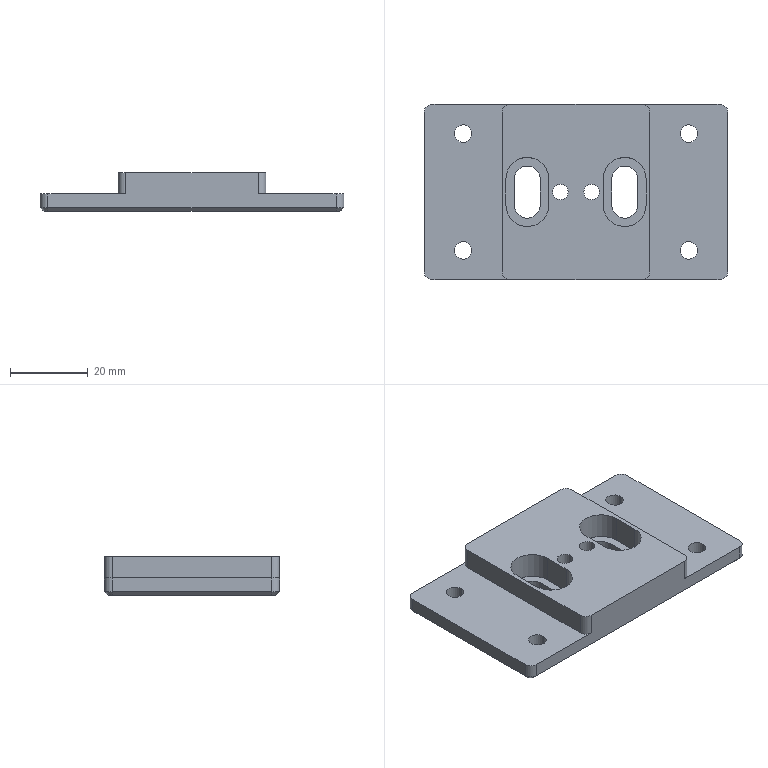NC program | NX | posted with a generic post | part box 78 x 45 x 10 mm
Lines 1 to 1682 of 4289, first 1506 of 1672 lines:
N10 G17 G21 G94 G90
(FLOOR_WALL , TOOL : D63)
N12 T01 M6
N14 G54
N16 G17 G0 G90 X-76.5 Y0. S6500 M3
N18 G43 Z30. H1
N20 Z3.
N22 G94 G1 Z0. F1250.
N24 X-73.5
N26 X73.5
N28 X76.5
N30 Z3.
N32 G0 Z30.
N34 M5
(ADAPTIVE_MILLING , TOOL : D10)
N36 T10 M6
N38 G54
N40 G17 G0 G90 X-49.696 Y-0.05 S9500 M3
N42 G43 Z30. H10
N44 Z-9.
N46 G94 G1 Z-10. F1000.
N48 X-48.34 Y-0.58 F3000.
N50 G3 X-47.049 Y-0.05 R1.015
N52 X-46.406 Y3.11 R9.424
N54 X-46.21 Y14.606 R185.073
N56 G2 X-46.176 Y23.305 R429.662
N58 X-43.276 Y27.539 R6.067
N60 X-37.706 Y29.327 R13.136
N62 X-29.118 Y29.675 R79.661
N64 G1 X-27.618 Y29.682
N66 X-25.518 Y29.687
N68 X-21.918 Y29.69
N70 X-8.218 Y29.691
N72 X39.282
N74 X39.382 Y29.689
N76 G2 X43.858 Y27.028 R5.824
N78 X45.771 Y21.61 R12.335
N80 X46.17 Y13.325 R66.724
N82 G1 X46.178 Y12.025
N84 X46.184 Y10.325
N86 X46.188 Y7.825
N88 X46.19 Y2.725
N90 Y-22.775
N92 Y-22.875
N94 G2 X43.535 Y-27.355 R5.815
N96 X38.118 Y-29.271 R12.321
N98 X30.134 Y-29.668 R64.412
N100 G1 X28.934 Y-29.676
N102 X27.334 Y-29.683
N104 X25.134 Y-29.687
N106 X21.234 Y-29.69
N108 X-0.766 Y-29.691
N110 X-39.266
N112 G2 X-43.609 Y-27.362 R5.645
N114 X-45.71 Y-22.022 R11.517
N116 X-46.166 Y-13.843 R57.666
N118 X-46.15 Y-2.344 R358.837
N120 G3 X-45.434 Y11.629 R117.265
N122 G1 X-45.426 Y13.229
N124 X-45.421 Y15.429
N126 X-45.418 Y18.929
N128 X-45.417 Y20.029
N130 X-45.414 Y20.229
N132 X-45.406 Y20.429
N134 X-45.4 Y20.529
N136 X-45.393 Y20.629
N138 G2 X-41.395 Y26.625 R7.729
N140 X-35.115 Y28.496 R16.062
N142 X-25.726 Y28.865 R92.161
N144 G1 X-24.226 Y28.872
N146 X-22.127 Y28.877
N148 X-18.827 Y28.88
N150 X-10.427 Y28.882
N152 X36.473
N154 X36.673 Y28.88
N156 G2 X42.939 Y25.168 R7.555
N158 X44.964 Y18.84 R15.167
N160 X45.363 Y9.553 R83.82
N162 G1 X45.37 Y8.053
N164 X45.376 Y6.053
N166 X45.38 Y3.053
N168 X45.381 Y-3.547
N170 X45.382 Y-20.047
N172 X45.381 Y-20.147
N174 G2 X41.606 Y-26.479 R7.587
N176 X35.465 Y-28.45 R15.175
N178 X25.98 Y-28.863 R83.109
N180 G1 X24.48 Y-28.87
N182 X22.48 Y-28.876
N184 X19.38 Y-28.88
N186 X12.88 Y-28.882
N188 X-36.52
N190 X-36.62 Y-28.881
N192 G2 X-42.965 Y-25.128 R7.577
N194 X-44.973 Y-18.793 R15.322
N196 X-45.363 Y-9.507 R85.57
N198 X-44.961 Y1.679 R97.942
N200 G3 X-44.625 Y17.873 R263.26
N202 G2 X-44.092 Y21.014 R9.947
N204 G1 X-43.977 Y22.032
N206 X-43.951 Y22.147
N208 G2 X-41.5 Y26.048 R7.672
N210 X-38.532 Y27.477 R8.031
N212 X-29.579 Y27.987 R94.219
N214 X-10.679 Y28.073 R882.599
N216 G1 X34.221
N218 X34.421 Y28.07
N220 X34.621 Y28.066
N222 X34.821 Y28.058
N224 X34.92 Y28.053
N226 G2 X37.322 Y27.614 R10.194
N228 X40.152 Y26.911 R7.665
N230 X43.411 Y23.652 R7.672
N232 X44.147 Y20.529 R8.254
N234 X44.569 Y2.779 R255.07
N236 G1 X44.572 Y-1.521
N238 X44.573 Y-15.521
N240 Y-17.721
N242 X44.57 Y-17.921
N244 X44.566 Y-18.121
N246 X44.558 Y-18.32
N248 G2 X44.115 Y-20.813 R10.023
N250 X43.411 Y-23.652 R7.679
N252 X40.152 Y-26.911 R7.672
N254 X37.029 Y-27.647 R8.254
N256 X21.179 Y-28.065 R231.381
N258 G1 X18.379 Y-28.07
N260 X13.379 Y-28.073
N262 X-25.221
N264 X-34.221
N266 X-34.421 Y-28.07
N268 X-34.621 Y-28.066
N270 G2 X-37.314 Y-27.615 R9.926
N272 X-40.152 Y-26.911 R7.678
N274 X-43.411 Y-23.652 R7.672
N276 X-44.147 Y-20.529 R8.254
N278 X-44.434 Y-2.882 R158.962
N280 G1 X-44.393 Y-2.183
N282 X-44.326 Y-1.085
N284 X-44.275 Y-0.287
N286 X-44.223 Y0.612
N288 X-44.157 Y1.81
N290 X-44.15 Y1.934
N292 Y20.471
N294 X-44.147 Y20.529
N296 X-44.091 Y21.026
N298 X-44.033 Y21.588
N300 X-43.951 Y22.147
N302 G2 X-41.5 Y26.048 R7.672
N304 X-38.532 Y27.477 R8.031
N306 G1 X-36.971 Y27.65
N308 X36.971
N310 X37.029 Y27.647
N312 X37.327 Y27.613
N314 G2 X40.152 Y26.911 R7.657
N316 X43.411 Y23.652 R7.672
N318 G1 X43.461 Y23.547
N320 X43.951 Y22.147
N322 X43.977 Y22.032
N324 X44.15 Y20.471
N326 Y-20.471
N328 X44.147 Y-20.529
N330 X44.113 Y-20.827
N332 G2 X43.411 Y-23.652 R7.657
N334 X40.152 Y-26.911 R7.672
N336 G1 X40.047 Y-26.961
N338 X38.647 Y-27.451
N340 X38.532 Y-27.477
N342 X36.971 Y-27.65
N344 X-36.971
N346 X-37.029 Y-27.647
N348 X-37.327 Y-27.613
N350 G2 X-40.152 Y-26.911 R7.657
N352 X-43.411 Y-23.652 R7.672
N354 G1 X-43.461 Y-23.547
N356 X-43.951 Y-22.147
N358 X-43.977 Y-22.032
N360 X-44.15 Y-20.471
N362 Y2.029
N364 G3 X-45.004 Y3.027 R1.016
N366 G1 X-46.57 Y3.271
N368 Z-7.
N370 G0 Z30.
N372 X-17.027 Y-30.147
N374 Z-4.349
N376 G1 Z-5.349 F1000.
N378 X-16.915 Y-29.348 F3000.
N380 X-16.827 Y-28.545
N382 G3 X-17.723 Y-27.569 R1.015
N384 G2 X-19.815 Y-27.183 R16.236
N386 G3 X-27.301 Y-26.829 R57.109
N388 G2 X-35.5 Y-26.768 R358.172
N390 X-41.868 Y-22.187 R7.175
N392 X-43.108 Y-16.042 R18.598
N394 X-43.29 Y-2.345 R262.741
N396 G1 X-43.291 Y10.755
N398 Y17.855
N400 X-43.288 Y18.155
N402 X-43.281 Y18.455
N404 X-43.274 Y18.655
N406 G2 X-38.625 Y25.388 R7.203
N408 X-32.576 Y26.607 R18.677
N410 X-20.479 Y26.805 R249.647
N412 G1 X-20.381 Y26.824
N414 X-20.285 Y26.852
N416 X-20.191 Y26.886
N418 X-20.152 Y26.911
N420 X-20.047 Y26.961
N422 X-18.647 Y27.451
N424 X-18.532 Y27.477
N426 X-17.638 Y27.578
N428 G3 X-17.737 Y29.573 R1.001
N430 G1 X-19.732 Y29.708 Z-5.249
N432 X-21.535 Y29.828
N434 X-30.91
N436 G3 X-37.067 Y29.07 R25.605
N438 G1 X-39.365 Y28.483
N440 G3 X-42.229 Y27.036 R8.814
N442 G1 X-42.693 Y26.628
N444 X-43.125 Y26.186
N446 X-44.628 Y24.467
N448 G3 X-45.923 Y21.531 R6.624
N450 X-46.251 Y17.815 R23.796
N452 G1 X-46.469 Y-12.529
N454 G3 X-45.306 Y-21.924 R37.581
N456 X-42.558 Y-26.649 R10.739
N458 G1 X-41.378 Y-27.811
N460 G3 X-38.52 Y-29.278 R6.575
N462 X-34.822 Y-29.815 R23.711
N464 G1 X-21.829 Y-30.633
N466 X-21.59 Y-30.616
N468 X-21.36 Y-30.549
N470 X-19.622 Y-29.777
N472 X-19.017 Y-29.513 Z-5.282
N474 X-18.422 Y-29.227 Z-5.315
N476 G3 X-18.023 Y-28.694 Z-5.349 R1.039
N478 X-18.647 Y-27.451 R1.005
N480 X-24.663 Y-26.187 R16.875
N482 X-33.56 Y-25.986 R419.368
N484 G2 X-40.311 Y-21.648 R8.075
N486 X-42.123 Y-15.246 R16.696
N488 X-42.473 Y-4.356 R113.695
N490 G1 X-42.478 Y-2.156
N492 X-42.481 Y1.544
N494 X-42.482 Y12.844
N496 Y15.944
N498 X-42.48 Y16.144
N500 X-42.478 Y16.344
N502 G2 X-37.96 Y23.901 R8.152
N504 X-31.436 Y25.655 R17.356
N506 X-22.245 Y25.989 R121.545
N508 G3 X-21.366 Y26.148 R2.601
N510 G1 X-20.181 Y26.893
N512 G3 X-19.876 Y28.287 R1.004
N514 X-20.781 Y28.754 Z-5.296 R1.115
N516 G1 X-21.714 Y28.866 Z-5.249
N518 X-24.078 Y29.143
N520 X-27.576 Y29.128
N522 G3 X-31.55 Y28.771 R34.824
N524 G1 X-34.142 Y28.367
N526 G3 X-38.741 Y26.858 R17.997
N528 G1 X-39.56 Y26.412
N530 X-40.354 Y25.922
N532 X-41.525 Y25.151
N534 X-42.68 Y24.357
N536 G3 X-43.753 Y22.981 R4.397
N538 G1 X-44.211 Y21.983
N540 X-44.643 Y20.975
N542 G3 X-45.305 Y17.878 R10.422
N544 G1 X-45.55 Y13.201
N546 X-45.736 Y8.52
N548 X-46.049 Y-1.477
N550 G3 X-45.387 Y-13.915 R74.276
N552 G1 X-44.7 Y-18.867
N554 G3 X-43.334 Y-22.574 R9.795
N556 G1 X-42.783 Y-23.403
N558 X-41.307 Y-25.411
N560 G3 X-40.231 Y-26.531 R6.738
N562 X-37.274 Y-28.244 R14.155
N564 X-34.876 Y-28.858 R9.068
N566 G1 X-23.229 Y-30.143
N568 G3 X-22.68 Y-30.048 R1.055
N570 G1 X-21.077 Y-29.266
N572 X-20.481 Y-28.981 Z-5.282
N574 X-19.897 Y-28.674 Z-5.315
N576 G3 X-19.516 Y-28.128 Z-5.349 R1.039
N578 X-20.047 Y-26.961 R1.007
N580 X-23.812 Y-25.676 R8.467
N582 X-31.295 Y-25.249 R69.666
N584 G2 X-39.48 Y-20.075 R9.177
N586 X-41.301 Y-13.256 R18.936
N588 X-41.661 Y-2.366 R118.207
N590 X-41.64 Y15.333 R923.775
N592 X-36.575 Y22.959 R9.056
N594 X-29.763 Y24.798 R18.711
N596 X-23.176 Y25.191 R200.74
N598 G3 X-21.5 Y26.048 R2.091
N600 G1 X-21.408 Y26.121
N602 X-21.323 Y26.175
N604 G3 X-21.009 Y27.553 R1.004
N606 X-21.92 Y28.036 Z-5.295 R1.109
N608 G1 X-22.838 Y28.146 Z-5.249
N610 X-25.22 Y28.425
N612 X-26.344 Y28.426
N614 X-27.466 Y28.385
N616 X-28.209 Y28.3
N618 X-28.946 Y28.18
N620 X-31.459 Y27.681
N622 X-33.967 Y27.161
N624 G3 X-38.298 Y25.602 R22.076
N626 X-41.392 Y23.152 R9.534
N628 G1 X-42.312 Y22.023
N630 X-43.214 Y20.88
N632 G3 X-44.07 Y19.032 R5.959
N634 X-44.547 Y15.96 R16.463
N636 G1 X-44.67 Y14.092
N638 X-44.736 Y12.222
N640 X-45.007 Y-5.279
N642 G3 X-44.37 Y-13.971 R49.652
N644 G1 X-43.942 Y-16.521
N646 G3 X-42.484 Y-21.098 R21.242
N648 X-39.929 Y-24.623 R11.844
N650 G1 X-38.65 Y-25.812
N652 G3 X-36.084 Y-27.305 R9.328
N654 X-32.213 Y-28.203 R13.677
N656 G1 X-24.454 Y-28.845
N658 X-22.235 Y-28.575
N660 X-21.57 Y-28.497 Z-5.283
N662 X-20.908 Y-28.397 Z-5.316
N664 G3 X-20.379 Y-28.021 Z-5.349 R1.041
N666 X-20.66 Y-26.591 R1.004
N668 X-25.088 Y-24.933 R9.128
N670 X-30.566 Y-24.46 R108.938
N672 G2 X-38.695 Y-18.59 R10.05
N674 X-40.481 Y-11.551 R20.915
N676 X-40.847 Y-0.961 R119.577
N678 X-40.828 Y13.639 R749.065
N680 X-35.279 Y22.066 R9.806
N682 X-28.071 Y23.977 R20.186
N684 G3 X-23.597 Y24.439 R61.952
N686 X-22.548 Y25. R1.508
N688 G1 X-21.983 Y25.565
N690 G3 X-21.811 Y26.749 R1.007
N692 X-22.687 Y27.289 Z-5.295 R1.11
N694 G1 X-23.598 Y27.46 Z-5.249
N696 X-25.626 Y27.833
N698 X-25.88 Y27.815
N700 X-29.005 Y27.196
N702 X-32.126 Y26.552
N704 G3 X-37.733 Y24.215 R18.405
N706 X-41.371 Y20.86 R14.166
N708 X-43.398 Y16.387 R9.938
N710 X-43.956 Y12.064 R33.416
N712 X-44.196 Y4.204 R96.24
N714 G1 X-44.158 Y2.707
N716 X-43.745 Y-9.164
N718 G3 X-42.963 Y-15.338 R34.55
N720 G1 X-42.714 Y-16.469
N722 X-42.419 Y-17.588
N724 G3 X-40.984 Y-20.659 R13.498
N726 X-38.929 Y-23.511 R23.056
N728 X-34.108 Y-26.687 R11.409
N730 G1 X-33.152 Y-26.973
N732 X-32.183 Y-27.209
N734 X-30.81 Y-27.492
N736 X-29.429 Y-27.734
N738 X-25.305 Y-28.371
N740 X-25. Y-28.372
N742 X-23.018 Y-28.067
N744 X-22.364 Y-27.971 Z-5.282
N746 X-21.715 Y-27.852 Z-5.315
N748 G3 X-21.189 Y-27.443 Z-5.349 R1.039
N750 X-21.408 Y-26.121 R1.005
N752 X-24.384 Y-24.546 R5.831
N754 X-29.222 Y-23.792 R43.916
N756 G2 X-37.913 Y-17.225 R10.96
N758 X-39.716 Y-9.471 R23.407
N760 X-40.047 Y3.221 R166.788
N762 X-39.993 Y12.419 R204.804
N764 X-33.895 Y21.278 R10.435
N766 X-27.467 Y23.062 R21.125
N768 G3 X-23.741 Y23.771 R19.944
N770 X-23.049 Y24.227 R1.57
N772 G1 X-22.624 Y24.904
N774 G3 X-22.583 Y25.898 R1.014
N776 X-23.301 Y26.427 Z-5.303 R1.049
N778 G1 X-24.341 Y26.712 Z-5.249
N780 X-26.109 Y27.187
N782 X-26.316 Y27.188
N784 X-26.521 Y27.154
N786 G3 X-30.978 Y25.741 R69.932
N788 G1 X-32.58 Y25.122
N790 X-34.175 Y24.486
N792 G3 X-38.369 Y21.861 R17.493
N794 X-41.461 Y18.249 R12.617
N796 X-42.583 Y15.188 R11.04
N798 X-42.98 Y12.104 R18.094
N800 G1 X-43.397 Y1.488
N802 G3 X-42.983 Y-8.471 R62.231
N804 G1 X-42.74 Y-10.432
N806 X-42.441 Y-12.386
N808 G3 X-41.108 Y-17.622 R43.62
N810 X-35.439 Y-24.718 R12.319
N812 X-32.897 Y-25.872 R16.542
N814 G1 X-31.571 Y-26.33
N816 X-30.229 Y-26.74
N818 X-25.68 Y-28.016
N820 X-25.448 Y-28.048
N822 X-25.215 Y-28.034
N824 X-23.424 Y-27.678
N826 X-22.776 Y-27.554 Z-5.282
N828 X-22.132 Y-27.407 Z-5.315
N830 G3 X-21.625 Y-26.975 Z-5.349 R1.039
N832 X-21.782 Y-25.766 R1.007
N834 X-25.109 Y-23.855 R6.221
N836 G2 X-29.399 Y-22.885 R291.286
N838 X-37.231 Y-15.726 R11.907
N840 X-38.909 Y-7.938 R25.813
N842 X-39.237 Y4.755 R174.442
N844 X-39.135 Y11.452 R80.404
N846 X-32.778 Y20.395 R10.909
N848 X-26.672 Y22.251 R25.621
N850 G3 X-23.822 Y23.153 R10.905
N852 X-23.411 Y23.652 R1.541
N854 G1 X-23.038 Y24.245
N856 G3 X-23.167 Y25.473 R1.007
N858 X-24.087 Y25.761 Z-5.299 R1.037
N860 G1 X-25.079 Y25.659 Z-5.249
N862 X-26.233 Y25.544
N864 X-27.385 Y25.41
N866 X-29.021 Y25.002
N868 X-30.645 Y24.549
N870 G3 X-36.058 Y22.043 R21.755
N872 X-38.841 Y19.587 R13.102
N874 G1 X-40.311 Y17.835
N876 G3 X-41.474 Y15.434 R7.556
N878 G1 X-41.71 Y14.53
N880 X-41.889 Y13.613
N882 G3 X-42.385 Y8.164 R32.733
N884 G1 X-42.39 Y3.246
N886 X-42.37 Y-1.672
N888 G3 X-41.847 Y-8.932 R72.751
N890 G1 X-41.5 Y-11.615
N892 G3 X-40.078 Y-16.807 R23.581
N894 X-37.9 Y-20.548 R17.726
N896 X-32.097 Y-25.065 R13.364
N898 G1 X-26.245 Y-27.45
N900 G3 X-25.654 Y-27.501 R1.048
N902 G1 X-23.984 Y-27.134
N904 X-23.331 Y-26.996 Z-5.282
N906 X-22.683 Y-26.835 Z-5.316
N908 G3 X-22.19 Y-26.408 Z-5.349 R1.04
N910 X-22.348 Y-25.2 R1.007
N912 X-25.324 Y-23.284 R5.749
N914 G2 X-29.769 Y-21.768 R41.624
N916 X-36.592 Y-14.162 R13.057
N918 X-38.146 Y-5.936 R29.445
N920 X-38.367 Y9.557 R187.76
N922 X-31.819 Y19.472 R11.374
N924 X-26.749 Y21.308 R30.248
N926 G3 X-24.004 Y22.482 R9.19
N928 X-23.461 Y23.547 R2.228
N930 X-23.673 Y24.558 R1.011
N932 X-24.526 Y24.874 Z-5.302 R1.046
N934 G1 X-25.583 Y24.848 Z-5.249
N936 X-27.549 Y24.79
N938 X-27.808 Y24.711
N940 X-30.647 Y23.408
N942 X-33.478 Y22.088
N944 G3 X-37.357 Y19.405 R17.782
N946 X-39.031 Y17.25 R10.785
N948 X-40.513 Y14.124 R17.41
N950 X-41.089 Y11.444 R13.822
N952 X-41.759 Y3.778 R69.955
N954 X-41.645 Y-0.378 R44.213
N956 G1 X-41.354 Y-4.22
N958 X-41.044 Y-8.061
N960 G3 X-39.786 Y-14.202 R33.376
N962 X-37.127 Y-19.529 R18.595
N964 G1 X-36.447 Y-20.461
N966 X-35.727 Y-21.364
N968 G3 X-30.472 Y-24.857 R12.476
N970 G1 X-26.855 Y-26.105
N972 X-24.694 Y-26.324
N974 X-24.045 Y-26.394 Z-5.282
N976 X-23.393 Y-26.437 Z-5.314
N978 G3 X-22.773 Y-26.159 Z-5.349 R1.038
N980 X-22.621 Y-24.908 R1.007
N982 X-24.849 Y-22.984 R4.491
N984 G2 X-29.133 Y-21.054 R82.148
N986 X-35.88 Y-12.831 R14.312
N988 X-37.372 Y-4.085 R33.221
N990 X-37.529 Y8.509 R131.827
N992 X-31.207 Y18.413 R11.761
N994 X-26.263 Y20.573 R45.314
N996 G3 X-24.121 Y21.826 R6.281
N998 X-23.687 Y22.902 R4.923
N1000 X-23.935 Y23.95 R1.011
N1002 X-24.827 Y24.231 Z-5.301 R1.135
N1004 G1 X-25.861 Y24.222 Z-5.249
N1006 X-27.66 Y24.199
N1008 X-27.852 Y24.148
N1010 X-28.034 Y24.066
N1012 X-30.484 Y22.601
N1014 X-32.924 Y21.118
N1016 G3 X-37.373 Y17.197 R21.29
N1018 X-39.142 Y14.3 R12.771
N1020 X-40.463 Y10.289 R18.335
N1022 X-40.683 Y7.82 R13.498
N1024 G1 X-40.608 Y-2.805
N1026 G3 X-39.795 Y-10.221 R36.9
N1028 G1 X-39.514 Y-11.527
N1030 X-39.186 Y-12.822
N1032 G3 X-36.027 Y-19.135 R18.99
N1034 X-31.123 Y-23.411 R16.313
N1036 G1 X-27.287 Y-25.565
N1038 X-27.088 Y-25.646
N1040 X-26.877 Y-25.69
N1042 X-25.008 Y-25.838
N1044 X-24.353 Y-25.896 Z-5.282
N1046 X-23.696 Y-25.928 Z-5.315
N1048 G3 X-23.087 Y-25.646 Z-5.349 R1.039
N1050 X-22.941 Y-24.4 R1.007
N1052 X-25.17 Y-22.312 R5.279
N1054 G2 X-29.623 Y-19.637 R39.755
N1056 X-35.375 Y-10.849 R16.112
N1058 X-36.63 Y-1.554 R41.35
N1060 X-36.682 Y7.542 R87.595
N1062 X-30.562 Y17.413 R12.271
N1064 X-25.958 Y19.827 R78.966
N1066 G3 X-24.153 Y21.216 R5.
N1068 X-23.955 Y22.13 R3.206
N1070 X-24.402 Y23.202 R1.007
N1072 X-25.363 Y23.259 Z-5.299 R1.037
N1074 G1 X-26.302 Y22.921 Z-5.249
N1076 X-28.305 Y22.199
N1078 X-28.455 Y22.13
N1080 X-29.923 Y21.307
N1082 X-31.37 Y20.449
N1084 G3 X-35.628 Y17.2 R30.221
N1086 X-38.354 Y13.086 R10.962
N1088 X-39.439 Y8.893 R16.044
N1090 G1 X-39.907 Y4.547
N1092 X-40.004 Y3.302
N1094 X-40.042 Y2.055
N1096 X-40.017 Y1.432
N1098 X-39.976 Y0.809
N1100 X-39.617 Y-3.056
N1102 X-39.237 Y-6.92
N1104 G3 X-37.902 Y-13.013 R34.9
N1106 X-35.574 Y-17.837 R17.228
N1108 X-32.505 Y-21.26 R18.589
N1110 G1 X-31.65 Y-21.987
N1112 X-30.768 Y-22.683
N1114 X-27.607 Y-25.057
N1116 G3 X-27.064 Y-25.255 R1.051
N1118 G1 X-25.316 Y-25.356
N1120 X-24.656 Y-25.399 Z-5.282
N1122 X-23.995 Y-25.418 Z-5.315
N1124 G3 X-23.397 Y-25.129 Z-5.349 R1.039
N1126 X-23.26 Y-23.892 R1.007
N1128 X-25.339 Y-21.645 R5.766
N1130 G2 X-29.926 Y-18.109 R34.106
N1132 X-34.801 Y-8.973 R18.311
N1134 X-35.871 Y0.953 R51.581
N1136 X-35.699 Y7.642 R37.584
N1138 X-30.3 Y16.19 R12.703
N1140 X-25.816 Y19.011 R103.195
N1142 G3 X-24.207 Y20.482 R4.979
N1144 X-24.022 Y21.637 R5.423
N1146 X-24.525 Y22.62 R1.01
N1148 X-25.409 Y22.674 Z-5.303 R1.049
N1150 G1 X-26.443 Y22.349 Z-5.249
N1152 X-28.221 Y21.791
N1154 X-28.376 Y21.723
N1156 X-28.522 Y21.637
N1158 X-33.024 Y18.26
N1160 G3 X-36.831 Y13.552 R12.433
N1162 X-38.83 Y7.587 R24.313
N1164 X-39.141 Y3.35 R19.584
N1166 G1 X-38.951 Y-1.468
N1168 G3 X-37.503 Y-10.667 R51.208
N1170 X-34.38 Y-17.544 R22.835
N1172 G1 X-33.611 Y-18.612
N1174 X-32.825 Y-19.667
N1176 G3 X-29.889 Y-22.307 R12.475
N1178 G1 X-27.874 Y-23.597
N1180 X-25.82 Y-24.4
N1182 X-25.215 Y-24.641 Z-5.282
N1184 X-24.6 Y-24.858 Z-5.314
N1186 G3 X-23.926 Y-24.755 Z-5.349 R1.038
N1188 X-23.461 Y-23.547 R1.006
N1190 X-25.046 Y-21.287 R4.825
N1192 G2 X-29.12 Y-17.596 R61.317
N1194 X-34.108 Y-7.514 R20.263
N1196 X-34.975 Y5.524 R54.962
N1198 X-29.682 Y15.237 R13.473
N1200 X-25.573 Y18.255 R540.304
N1202 G3 X-24.224 Y19.71 R4.816
N1204 X-24.113 Y20.827 R6.496
N1206 X-24.608 Y21.806 R1.01
N1208 X-25.483 Y21.871 Z-5.304 R1.051
N1210 G1 X-26.533 Y21.564 Z-5.249
N1212 X-28.187 Y21.08
N1214 X-28.414 Y20.977
N1216 X-28.613 Y20.827
N1218 X-33.474 Y15.966
N1220 G3 X-37.663 Y7.814 R14.761
N1222 G1 X-37.79 Y6.891
N1224 X-37.873 Y5.963
N1226 X-38.103 Y1.776
N1228 G3 X-37.766 Y-4.615 R38.997
N1230 X-37.155 Y-8.308 R42.153
N1232 X-35.826 Y-12.724 R33.038
N1234 X-32.826 Y-17.868 R19.631
N1236 G1 X-31.617 Y-19.297
N1238 X-30.363 Y-20.688
N1240 X-28.127 Y-23.075
N1242 X-27.944 Y-23.224
N1244 X-27.735 Y-23.332
N1246 X-25.974 Y-23.964
N1248 X-25.361 Y-24.189 Z-5.282
N1250 X-24.741 Y-24.39 Z-5.314
N1252 G3 X-24.071 Y-24.271 Z-5.349 R1.038
N1254 X-23.627 Y-23.075 R1.007
N1256 X-25.365 Y-20.313 R6.434
N1258 G2 X-29.493 Y-15.696 R44.517
N1260 X-33.502 Y-5.561 R23.486
N1262 X-34.086 Y4.7 R44.881
N1264 X-29.241 Y14.162 R14.154
N1266 G1 X-25.285 Y17.534
N1268 G3 X-24.192 Y18.945 R4.197
N1270 X-24.15 Y20.065 R7.43
N1272 X-24.884 Y21.029 R1.007
N1274 X-25.882 Y20.77 Z-5.295 R1.109
N1276 G1 X-26.635 Y20.232 Z-5.249
N1278 X-28.073 Y19.201
N1280 X-29.537 Y18.207
N1282 G3 X-31.423 Y16.593 R10.707
N1284 G1 X-33.445 Y14.38
N1286 G3 X-35.697 Y10.526 R12.964
N1288 X-36.866 Y6.34 R20.982
N1290 G1 X-37.172 Y4.491
N1292 X-37.446 Y2.637
N1294 G3 X-37.46 Y1.394 R6.405
N1296 G1 X-37.201 Y-1.28
N1298 X-36.924 Y-3.952
N1300 G3 X-35.507 Y-10.271 R32.676
N1302 X-31.569 Y-18.023 R31.925
N1304 G1 X-30.485 Y-19.548
N1306 X-28.358 Y-22.414
N1308 G3 X-27.874 Y-22.766 R1.047
N1310 G1 X-26.207 Y-23.326
N1312 X-25.585 Y-23.541 Z-5.282
N1314 X-24.955 Y-23.732 Z-5.315
N1316 G3 X-24.297 Y-23.608 Z-5.349 R1.039
N1318 X-23.858 Y-22.414 R1.007
N1320 X-25.384 Y-19.525 R6.907
N1322 G2 X-29.235 Y-14.42 R51.901
N1324 X-32.788 Y-4.094 R26.595
N1326 X-33.15 Y4.178 R34.189
N1328 X-28.737 Y13.152 R14.915
N1330 G3 X-25.084 Y16.709 R333.833
N1332 X-24.163 Y18.116 R3.423
N1334 G1 X-24.15 Y18.215
N1336 Y19.215
N1338 G3 X-24.876 Y20.177 R1.007
N1340 X-25.879 Y19.924 Z-5.295 R1.108
N1342 G1 X-26.631 Y19.391 Z-5.249
N1344 X-28.368 Y18.159
N1346 X-28.497 Y18.05
N1348 X-30.076 Y16.476
N1350 X-31.639 Y14.887
N1352 G3 X-34.457 Y10.678 R17.13
N1354 X-36.107 Y6.21 R24.462
N1356 X-36.45 Y1.292 R15.203
N1358 X-35.37 Y-7.163 R63.822
N1360 X-33.79 Y-12.37 R34.132
N1362 X-30.823 Y-17.551 R23.556
N1364 G1 X-28.324 Y-20.868
N1366 X-28.118 Y-21.072
N1368 X-26.46 Y-22.291
N1370 X-25.438 Y-23.028 Z-5.312
N1372 G3 X-24.721 Y-23.113 Z-5.349 R1.03
N1374 X-23.977 Y-22.032 R1.005
N1376 X-25.096 Y-19.077 R5.876
N1378 G2 X-28.552 Y-13.812 R99.192
N1380 X-32.1 Y-2.332 R29.86
N1382 X-31.914 Y5.228 R22.095
N1384 X-27.977 Y12.433 R16.422
N1386 G3 X-24.702 Y16.075 R81.666
N1388 X-24.15 Y17.152 R2.377
N1390 G1 Y18.252
N1392 G3 X-24.863 Y19.21 R1.007
N1394 X-25.871 Y18.969 Z-5.295 R1.107
N1396 G1 X-26.626 Y18.446 Z-5.249
N1398 X-28.266 Y17.31
N1400 X-28.387 Y17.205
N1402 X-28.497 Y17.088
N1404 X-30.377 Y14.592
N1406 X-32.236 Y12.08
N1408 G3 X-33.926 Y8.777 R15.685
N1410 X-34.978 Y5.449 R20.82
N1412 G1 X-35.099 Y4.712
N1414 X-35.181 Y3.97
N1416 X-35.31 Y2.26
N1418 X-35.387 Y0.548
N1420 G3 X-34.912 Y-4.714 R26.782
N1422 X-31.654 Y-14.43 R35.304
N1424 G1 X-31.003 Y-15.673
N1426 X-30.324 Y-16.902
N1428 X-28.391 Y-20.272
N1430 X-28.262 Y-20.442
N1432 X-28.105 Y-20.588
N1434 X-26.476 Y-21.75
N1436 X-25.985 Y-22.105 Z-5.279
N1438 X-25.484 Y-22.443 Z-5.31
N1440 G3 X-24.717 Y-22.495 Z-5.349 R1.027
N1442 X-24.045 Y-21.436 R1.007
N1444 X-25.189 Y-17.945 R7.442
N1446 G2 X-28.571 Y-11.821 R74.835
N1448 X-31.338 Y1.881 R30.838
N1450 X-27.71 Y11.134 R16.386
N1452 G3 X-24.596 Y15.044 R139.329
N1454 X-24.15 Y16.007 R2.281
N1456 G1 Y17.207
N1458 G3 X-24.849 Y18.161 R1.007
N1460 X-25.861 Y17.934 Z-5.295 R1.106
N1462 G1 X-26.622 Y17.421 Z-5.249
N1464 X-27.473 Y16.852
N1466 X-28.313 Y16.267
N1468 X-28.497 Y16.043
N1470 X-31.767 Y10.572
N1472 G3 X-33.563 Y6.731 R30.38
N1474 X-34.373 Y1.844 R13.563
N1476 X-34.207 Y-1.889 R33.298
N1478 X-33.757 Y-5.35 R40.704
N1480 X-32.037 Y-11.269 R34.305
N1482 G1 X-31.513 Y-12.571
N1484 X-30.961 Y-13.862
N1486 X-28.493 Y-19.365
N1488 G3 X-28.137 Y-19.787 R1.056
N1490 G1 X-26.479 Y-20.896
N1492 X-25.569 Y-21.491 Z-5.303
N1494 G3 X-24.689 Y-21.475 Z-5.349 R1.016
N1496 X-24.147 Y-20.529 R1.01
N1498 X-24.942 Y-17.303 R6.725
N1500 G2 X-27.856 Y-11.271 R152.261
N1502 X-30.385 Y0.681 R30.386
N1504 X-27.132 Y10.188 R17.102
N1506 G3 X-24.378 Y14.116 R84.538
N1508 X-24.15 Y14.741 R2.15
N1510 G1 Y16.041
N1512 G3 X-24.835 Y16.99 R1.007
N1514 X-25.783 Y16.821 Z-5.299 R1.037
N1516 G1 X-26.617 Y16.273 Z-5.249
N1518 X-28.256 Y15.185
N1520 X-28.388 Y15.04
N1522 X-28.497 Y14.876
N1524 X-30.073 Y11.732
N1526 X-31.632 Y8.58
N1528 G3 X-33.39 Y2.364 R21.881
N1530 X-33.298 Y-2.483 R20.165
N1532 X-31.878 Y-8.669 R34.784
N1534 G1 X-28.497 Y-18.806
N1536 G3 X-28.074 Y-19.34 R1.038
N1538 G1 X-26.482 Y-20.323
N1540 X-25.542 Y-20.89 Z-5.304
N1542 G3 X-24.672 Y-20.849 Z-5.349 R1.016
N1544 X-24.15 Y-19.971 R1.011
N1546 X-24.903 Y-16.082 R8.266
N1548 G2 X-27.764 Y-9.044 R108.129
N1550 X-29.38 Y0.369 R27.399
N1552 X-26.449 Y9.39 R17.998
N1554 G3 X-24.244 Y12.963 R62.919
N1556 G1 X-24.208 Y13.056
N1558 X-24.18 Y13.152
N1560 X-24.16 Y13.25
N1562 X-24.15 Y13.341
N1564 Y14.741
N1566 G3 X-25.192 Y15.74 R1.004
N1568 X-26.065 Y15.186 Z-5.295 R1.108
N1570 G1 X-26.611 Y14.443 Z-5.249
N1572 X-28.047 Y12.491
N1574 X-29.49 Y10.301
N1576 G3 X-32.073 Y3.474 R19.113
N1578 X-32.479 Y0.507 R26.408
N1580 X-32.36 Y-2.101 R14.117
N1582 X-31.575 Y-6.391 R32.48
N1584 X-30.122 Y-11.159 R41.901
N1586 G1 X-28.047 Y-16.721
N1588 X-27.909 Y-16.973
N1590 X-26.482 Y-18.866
N1592 X-26.169 Y-19.284 Z-5.275
N1594 X-25.843 Y-19.692 Z-5.301
N1596 G3 X-24.961 Y-19.953 Z-5.349 R1.015
N1598 X-24.15 Y-18.971 R1.007
N1600 X-24.918 Y-14.473 R10.483
N1602 G2 X-27.515 Y-6.805 R84.656
N1604 X-28.216 Y1.71 R21.734
N1606 X-25.502 Y9.077 R20.758
N1608 G3 X-24.188 Y11.547 R31.254
N1610 X-24.15 Y13.35 R14.343
N1612 X-25.173 Y14.35 R1.004
N1614 X-26.011 Y13.869 Z-5.299 R1.037
N1616 G1 X-26.605 Y13.072 Z-5.249
N1618 X-27.998 Y11.194
N1620 G3 X-30.271 Y5.941 R73.312
N1622 X-31.412 Y-1.383 R17.707
N1624 X-30.103 Y-8.734 R32.663
N1626 G1 X-28.006 Y-15.632
N1628 X-27.885 Y-15.838
N1630 X-26.487 Y-17.668
N1632 X-26.169 Y-18.087 Z-5.275
N1634 X-25.839 Y-18.495 Z-5.302
N1636 G3 X-24.962 Y-18.753 Z-5.349 R1.015
N1638 X-24.15 Y-17.771 R1.007
N1640 X-24.952 Y-12.467 R13.6
N1642 G2 X-27.063 Y-4.654 R59.495
N1644 X-25.193 Y7.579 R19.292
N1646 G3 X-24.163 Y9.853 R20.929
N1648 G1 X-24.15 Y9.952
N1650 Y11.752
N1652 G3 X-25.148 Y12.752 R1.005
N1654 X-26.006 Y12.279 Z-5.298 R1.035
N1656 G1 X-26.597 Y11.5 Z-5.249
N1658 X-27.895 Y9.791
N1660 X-27.979 Y9.651
N1662 X-28.047 Y9.502
N1664 X-28.754 Y7.386
N1666 X-29.447 Y5.265
N1668 G3 X-30.222 Y1.084 R20.852
N1670 G1 X-30.347 Y-0.472
N1672 X-30.439 Y-2.03
N1674 G3 X-30.332 Y-3.267 R5.599
N1676 G1 X-28.669 Y-11.216
N1678 X-28.352 Y-12.64
N1680 X-28.005 Y-14.058
N1682 X-27.863 Y-14.307
N1684 X-26.495 Y-16.069
N1686 X-26.171 Y-16.489 Z-5.276
N1688 X-25.835 Y-16.899 Z-5.302
N1690 G3 X-24.967 Y-17.154 Z-5.349 R1.015
N1692 X-24.15 Y-16.171 R1.007
N1694 X-24.842 Y-10.54 R16.784
N1696 G2 X-26.299 Y-3.295 R44.311
N1698 X-24.56 Y6.648 R20.596
N1700 G3 X-24.15 Y7.811 R8.308
N1702 G1 Y10.011
N1704 G3 X-25.114 Y11.01 R1.005
N1706 X-25.996 Y10.552 Z-5.297 R1.033
N1708 G1 X-26.589 Y9.795 Z-5.249
N1710 X-27.854 Y8.181
N1712 X-27.972 Y7.981
N1714 X-28.047 Y7.761
N1716 X-28.934 Y3.264
N1718 G3 X-29.008 Y-5.827 R28.679
N1720 G1 X-28.047 Y-12.121
N1722 G3 X-27.841 Y-12.592 R1.113
N1724 G1 X-26.501 Y-14.278
N1726 X-26.17 Y-14.697 Z-5.276
N1728 X-25.827 Y-15.106 Z-5.303
N1730 G3 X-24.964 Y-15.353 Z-5.349 R1.015
N1732 X-24.15 Y-14.371 R1.007
N1734 X-24.733 Y-8.016 R23.872
N1736 G2 X-25.282 Y0.033 R26.809
N1738 X-24.15 Y5.099 R30.657
N1740 G1 Y7.899
N1742 G3 X-25.252 Y8.997 R1.1
N1744 X-26.35 Y7.899 R1.1
N1746 G1 Y-12.071
N1748 G3 X-25.248 Y-13.169 R1.1
N1750 X-24.15 Y-12.071 R1.1
N1752 X-24.433 Y-4.781 R62.674
N1754 G2 X-24.15 Y1.019 R25.258
N1756 G1 Y5.119
N1758 G3 X-25.252 Y6.217 R1.1
N1760 X-26.35 Y5.119 R1.1
N1762 G1 Y-8.871
N1764 G3 X-25.248 Y-9.969 R1.1
N1766 X-24.15 Y-8.871 R1.1
N1768 G1 Y1.029
N1770 G3 X-25.004 Y2.027 R1.016
N1772 G1 X-26.565 Y2.272
N1774 Z-2.349
N1776 G0 Z30.
N1778 X17.027 Y30.147
N1780 Z-4.349
N1782 G1 Z-5.349 F1000.
N1784 X16.915 Y29.348 F3000.
N1786 X16.827 Y28.545
N1788 G3 X17.723 Y27.569 R1.015
N1790 G2 X19.717 Y27.2 R14.26
N1792 G3 X26.401 Y26.837 R49.215
N1794 G2 X35.6 Y26.76 R311.686
N1796 X41.917 Y22.101 R7.215
N1798 X43.103 Y16.146 R18.596
N1800 X43.289 Y4.25 R221.082
N1802 G1 X43.291 Y-1.45
N1804 Y-17.95
N1806 X43.289 Y-18.15
N1808 X43.282 Y-18.45
N1810 X43.275 Y-18.65
N1812 X43.265 Y-18.85
N1814 G2 X38.724 Y-25.348 R7.161
N1816 X32.383 Y-26.619 R18.737
N1818 X20.486 Y-26.803 R259.868
N1820 G1 X20.388 Y-26.822
N1822 X20.292 Y-26.849
N1824 X20.198 Y-26.883
N1826 X20.189 Y-26.888
N1828 X20.152 Y-26.911
N1830 X20.047 Y-26.961
N1832 X18.647 Y-27.451
N1834 X18.532 Y-27.477
N1836 X17.638 Y-27.578
N1838 G3 X17.737 Y-29.573 R1.001
N1840 G1 X19.732 Y-29.708 Z-5.249
N1842 X21.535 Y-29.828
N1844 X30.91
N1846 G3 X37.067 Y-29.07 R25.605
N1848 G1 X39.365 Y-28.483
N1850 G3 X42.229 Y-27.036 R8.814
N1852 G1 X42.693 Y-26.628
N1854 X43.125 Y-26.186
N1856 X44.628 Y-24.467
N1858 G3 X45.923 Y-21.531 R6.624
N1860 X46.251 Y-17.815 R23.796
N1862 G1 X46.469 Y12.529
N1864 G3 X45.306 Y21.924 R37.581
N1866 X42.558 Y26.649 R10.739
N1868 G1 X41.378 Y27.811
N1870 G3 X38.52 Y29.278 R6.575
N1872 X34.822 Y29.815 R23.711
N1874 G1 X21.829 Y30.633
N1876 X21.59 Y30.616
N1878 X21.36 Y30.549
N1880 X19.622 Y29.777
N1882 X19.017 Y29.513 Z-5.282
N1884 X18.422 Y29.227 Z-5.315
N1886 G3 X18.023 Y28.694 Z-5.349 R1.039
N1888 X18.647 Y27.451 R1.005
N1890 X24.863 Y26.176 R17.033
N1892 X33.66 Y25.978 R713.4
N1894 G2 X40.413 Y21.481 R8.107
N1896 X42.158 Y14.954 R17.437
N1898 X42.474 Y3.962 R126.657
N1900 G1 X42.479 Y1.562
N1902 X42.481 Y-2.738
N1904 X42.482 Y-15.938
N1906 X42.479 Y-16.238
N1908 X42.474 Y-16.538
N1910 X42.468 Y-16.738
N1912 G2 X38.06 Y-23.852 R8.072
N1914 X31.846 Y-25.611 R16.581
N1916 X22.357 Y-25.984 R105.557
N1918 G3 X21.37 Y-26.145 R2.861
N1920 G1 X20.184 Y-26.89
N1922 G3 X19.88 Y-28.284 R1.004
N1924 X20.784 Y-28.752 Z-5.296 R1.115
N1926 G1 X21.717 Y-28.864 Z-5.249
N1928 X24.082 Y-29.14
N1930 X27.58 Y-29.125
N1932 G3 X31.554 Y-28.769 R34.824
N1934 G1 X34.145 Y-28.365
N1936 G3 X38.745 Y-26.855 R17.997
N1938 G1 X39.564 Y-26.41
N1940 X40.358 Y-25.92
N1942 X41.528 Y-25.149
N1944 X42.684 Y-24.355
N1946 G3 X43.756 Y-22.978 R4.397
N1948 G1 X44.214 Y-21.981
N1950 X44.646 Y-20.972
N1952 G3 X45.308 Y-17.876 R10.422
N1954 G1 X45.554 Y-13.198
N1956 X45.739 Y-8.518
N1958 X46.053 Y1.479
N1960 G3 X45.39 Y13.917 R74.276
N1962 G1 X44.704 Y18.87
N1964 G3 X43.338 Y22.576 R9.795
N1966 G1 X42.787 Y23.406
N1968 X41.311 Y25.413
N1970 G3 X40.235 Y26.533 R6.738
N1972 X37.277 Y28.246 R14.153
N1974 X34.879 Y28.86 R9.065
N1976 G1 X23.229 Y30.143
N1978 G3 X22.681 Y30.048 R1.055
N1980 G1 X21.077 Y29.266
N1982 X20.481 Y28.981 Z-5.282
N1984 X19.897 Y28.674 Z-5.315
N1986 G3 X19.516 Y28.128 Z-5.349 R1.039
N1988 X20.047 Y26.961 R1.007
N1990 X23.91 Y25.66 R8.583
N1992 X31.494 Y25.238 R78.716
N1994 G2 X39.574 Y19.902 R9.19
N1996 X41.345 Y12.864 R19.823
N1998 X41.662 Y1.972 R132.758
N2000 X41.641 Y-15.328 R914.971
N2002 X36.583 Y-22.957 R9.041
N2004 X29.672 Y-24.808 R18.789
N2006 X23.184 Y-25.19 R212.927
N2008 G3 X21.5 Y-26.048 R2.094
N2010 G1 X21.408 Y-26.121
N2012 X21.323 Y-26.175
N2014 G3 X21.009 Y-27.553 R1.004
N2016 X21.92 Y-28.036 Z-5.295 R1.109
N2018 G1 X22.838 Y-28.146 Z-5.249
N2020 X25.22 Y-28.425
N2022 X26.344 Y-28.426
N2024 X27.466 Y-28.385
N2026 X28.209 Y-28.3
N2028 X28.946 Y-28.18
N2030 X31.459 Y-27.681
N2032 X33.967 Y-27.161
N2034 G3 X38.298 Y-25.602 R22.076
N2036 X41.392 Y-23.152 R9.534
N2038 G1 X42.312 Y-22.023
N2040 X43.214 Y-20.88
N2042 G3 X44.07 Y-19.032 R5.959
N2044 X44.547 Y-15.96 R16.463
N2046 G1 X44.67 Y-14.092
N2048 X44.736 Y-12.222
N2050 X45.007 Y5.279
N2052 G3 X44.37 Y13.971 R49.652
N2054 G1 X43.942 Y16.521
N2056 G3 X42.484 Y21.098 R21.242
N2058 X39.929 Y24.623 R11.844
N2060 G1 X38.65 Y25.812
N2062 G3 X36.084 Y27.305 R9.328
N2064 X32.213 Y28.203 R13.677
N2066 G1 X24.454 Y28.845
N2068 X22.235 Y28.575
N2070 X21.57 Y28.497 Z-5.283
N2072 X20.908 Y28.397 Z-5.316
N2074 G3 X20.379 Y28.021 Z-5.349 R1.041
N2076 X20.66 Y26.591 R1.004
N2078 X25.089 Y24.934 R9.157
N2080 X30.367 Y24.481 R87.821
N2082 G2 X38.741 Y18.502 R10.078
N2084 X40.505 Y11.354 R21.278
N2086 X40.852 Y-0.037 R135.395
N2088 X40.829 Y-13.636 R731.058
N2090 X35.195 Y-22.112 R9.823
N2092 X27.977 Y-23.986 R20.386
N2094 G3 X23.505 Y-24.458 R49.922
N2096 X22.548 Y-25. R1.41
N2098 G1 X21.983 Y-25.565
N2100 G3 X21.811 Y-26.749 R1.007
N2102 X22.687 Y-27.289 Z-5.295 R1.11
N2104 G1 X23.598 Y-27.46 Z-5.249
N2106 X25.626 Y-27.833
N2108 X25.88 Y-27.815
N2110 X29.005 Y-27.196
N2112 X32.126 Y-26.552
N2114 G3 X37.733 Y-24.215 R18.405
N2116 X41.371 Y-20.86 R14.166
N2118 X43.398 Y-16.387 R9.938
N2120 X43.956 Y-12.064 R33.416
N2122 X44.196 Y-4.204 R96.24
N2124 G1 X44.158 Y-2.707
N2126 X43.745 Y9.164
N2128 G3 X42.963 Y15.338 R34.55
N2130 G1 X42.714 Y16.469
N2132 X42.419 Y17.588
N2134 G3 X40.984 Y20.659 R13.498
N2136 X38.929 Y23.511 R23.056
N2138 X34.108 Y26.687 R11.409
N2140 G1 X33.152 Y26.973
N2142 X32.183 Y27.209
N2144 X30.81 Y27.492
N2146 X29.429 Y27.734
N2148 X25.305 Y28.371
N2150 X25. Y28.372
N2152 X23.018 Y28.067
N2154 X22.364 Y27.971 Z-5.282
N2156 X21.715 Y27.852 Z-5.315
N2158 G3 X21.189 Y27.443 Z-5.349 R1.039
N2160 X21.408 Y26.121 R1.005
N2162 X24.287 Y24.572 R5.737
N2164 X29.123 Y23.807 R39.601
N2166 G2 X37.915 Y17.227 R10.97
N2168 X39.706 Y9.573 R23.171
N2170 X40.043 Y-2.019 R147.644
N2172 X40. Y-12.318 R271.42
N2174 X33.987 Y-21.232 R10.415
N2176 X27.273 Y-23.092 R21.166
N2178 G3 X23.651 Y-23.807 R16.921
N2180 X23.048 Y-24.229 R1.538
N2182 G1 X22.622 Y-24.906
N2184 G3 X22.582 Y-25.899 R1.014
N2186 X23.299 Y-26.429 Z-5.303 R1.049
N2188 G1 X24.339 Y-26.714 Z-5.249
N2190 X26.107 Y-27.189
N2192 X26.315 Y-27.19
N2194 X26.52 Y-27.156
N2196 G3 X30.977 Y-25.743 R69.932
N2198 G1 X32.579 Y-25.125
N2200 X34.174 Y-24.488
N2202 G3 X38.367 Y-21.863 R17.493
N2204 X41.46 Y-18.252 R12.617
N2206 X42.582 Y-15.19 R11.04
N2208 X42.979 Y-12.106 R18.094
N2210 G1 X43.396 Y-1.49
N2212 G3 X42.981 Y8.469 R62.231
N2214 G1 X42.739 Y10.43
N2216 X42.44 Y12.384
N2218 G3 X41.107 Y17.62 R43.62
N2220 X35.438 Y24.716 R12.321
N2222 X32.896 Y25.87 R16.548
N2224 G1 X31.57 Y26.329
N2226 X30.228 Y26.739
N2228 X25.68 Y28.016
N2230 X25.448 Y28.048
N2232 X25.215 Y28.034
N2234 X23.424 Y27.678
N2236 X22.776 Y27.554 Z-5.282
N2238 X22.132 Y27.407 Z-5.315
N2240 G3 X21.625 Y26.975 Z-5.349 R1.039
N2242 X21.782 Y25.766 R1.007
N2244 X25.012 Y23.882 R6.102
N2246 G2 X29.398 Y22.883 R387.371
N2248 X37.271 Y15.634 R11.934
N2250 X38.9 Y8.037 R25.841
N2252 X39.236 Y-4.555 R166.091
N2254 X39.137 Y-11.452 R84.898
N2256 X32.871 Y-20.352 R10.882
N2258 X27.457 Y-22.082 R22.289
N2260 G3 X23.911 Y-23.101 R15.229
N2262 X23.411 Y-23.652 R1.312
N2264 G1 X23.038 Y-24.245
N2266 G3 X23.167 Y-25.473 R1.007
N2268 X24.087 Y-25.761 Z-5.299 R1.037
N2270 G1 X25.079 Y-25.659 Z-5.249
N2272 X26.233 Y-25.544
N2274 X27.385 Y-25.41
N2276 X29.021 Y-25.002
N2278 X30.645 Y-24.549
N2280 G3 X36.058 Y-22.043 R21.755
N2282 X38.841 Y-19.587 R13.102
N2284 G1 X40.311 Y-17.835
N2286 G3 X41.474 Y-15.434 R7.556
N2288 G1 X41.71 Y-14.53
N2290 X41.889 Y-13.613
N2292 G3 X42.385 Y-8.164 R32.733
N2294 G1 X42.39 Y-3.246
N2296 X42.37 Y1.672
N2298 G3 X41.847 Y8.932 R72.751
N2300 G1 X41.5 Y11.615
N2302 G3 X40.078 Y16.807 R23.581
N2304 X37.9 Y20.548 R17.726
N2306 X32.097 Y25.065 R13.364
N2308 G1 X26.245 Y27.45
N2310 G3 X25.654 Y27.501 R1.048
N2312 G1 X23.984 Y27.134
N2314 X23.331 Y26.996 Z-5.282
N2316 X22.683 Y26.835 Z-5.316
N2318 G3 X22.19 Y26.408 Z-5.349 R1.04
N2320 X22.348 Y25.2 R1.007
N2322 X25.135 Y23.35 R5.542
N2324 G2 X29.403 Y21.928 R64.836
N2326 X36.557 Y14.256 R13.
N2328 X38.133 Y6.136 R29.175
N2330 X38.367 Y-9.557 R186.873
N2332 X31.731 Y-19.518 R11.405
N2334 X26.654 Y-21.338 R32.001
N2336 G3 X23.93 Y-22.549 R8.043
N2338 X23.461 Y-23.547 R2.579
N2340 X23.673 Y-24.558 R1.011
N2342 X24.526 Y-24.874 Z-5.302 R1.046
N2344 G1 X25.583 Y-24.848 Z-5.249
N2346 X27.549 Y-24.79
N2348 X27.808 Y-24.711
N2350 X30.647 Y-23.408
N2352 X33.478 Y-22.088
N2354 G3 X37.357 Y-19.405 R17.782
N2356 X39.031 Y-17.25 R10.785
N2358 X40.513 Y-14.124 R17.41
N2360 X41.089 Y-11.444 R13.822
N2362 X41.759 Y-3.778 R69.955
N2364 X41.645 Y0.378 R44.213
N2366 G1 X41.354 Y4.22
N2368 X41.044 Y8.061
N2370 G3 X39.786 Y14.202 R33.376
N2372 X37.127 Y19.529 R18.595
N2374 G1 X36.447 Y20.461
N2376 X35.727 Y21.364
N2378 G3 X30.472 Y24.857 R12.476
N2380 G1 X26.855 Y26.105
N2382 X24.694 Y26.324
N2384 X24.045 Y26.394 Z-5.282
N2386 X23.393 Y26.437 Z-5.314
N2388 G3 X22.773 Y26.159 Z-5.349 R1.038
N2390 X22.621 Y24.908 R1.007
N2392 X24.848 Y22.982 R4.514
N2394 G2 X29.044 Y21.1 R90.768
N2396 X35.941 Y12.64 R14.338
N2398 X37.372 Y4.083 R33.895
N2400 X37.537 Y-8.411 R136.595
N2402 X30.943 Y-18.558 R11.844
N2404 X26.17 Y-20.613 R52.239
N2406 G3 X24.121 Y-21.828 R6.12
N2408 X23.687 Y-22.902 R4.882
N2410 X23.935 Y-23.95 R1.011
N2412 X24.827 Y-24.231 Z-5.301 R1.135
N2414 G1 X25.861 Y-24.222 Z-5.249
N2416 X27.66 Y-24.199
N2418 X27.852 Y-24.148
N2420 X28.034 Y-24.066
N2422 X30.484 Y-22.601
N2424 X32.924 Y-21.118
N2426 G3 X37.373 Y-17.197 R21.29
N2428 X39.142 Y-14.3 R12.771
N2430 X40.463 Y-10.289 R18.335
N2432 X40.683 Y-7.82 R13.498
N2434 G1 X40.608 Y2.805
N2436 G3 X39.795 Y10.221 R36.9
N2438 G1 X39.514 Y11.527
N2440 X39.186 Y12.822
N2442 G3 X36.027 Y19.135 R18.99
N2444 X31.123 Y23.411 R16.313
N2446 G1 X27.287 Y25.565
N2448 X27.088 Y25.646
N2450 X26.877 Y25.69
N2452 X25.008 Y25.838
N2454 X24.353 Y25.896 Z-5.282
N2456 X23.696 Y25.928 Z-5.315
N2458 G3 X23.087 Y25.646 Z-5.349 R1.039
N2460 X22.941 Y24.4 R1.007
N2462 X25.083 Y22.362 R5.126
N2464 G2 X29.542 Y19.696 R43.794
N2466 X35.345 Y10.944 R16.042
N2468 X36.609 Y1.952 R40.367
N2470 X36.682 Y-7.543 R86.948
N2472 X30.56 Y-17.413 R12.257
N2474 X25.87 Y-19.877 R84.465
N2476 G3 X24.152 Y-21.217 R4.785
N2478 X23.955 Y-22.13 R3.24
N2480 X24.402 Y-23.202 R1.007
N2482 X25.363 Y-23.259 Z-5.299 R1.037
N2484 G1 X26.302 Y-22.921 Z-5.249
N2486 X28.305 Y-22.199
N2488 X28.455 Y-22.13
N2490 X29.923 Y-21.307
N2492 X31.37 Y-20.449
N2494 G3 X35.628 Y-17.2 R30.221
N2496 X38.354 Y-13.086 R10.962
N2498 X39.439 Y-8.893 R16.044
N2500 G1 X39.907 Y-4.547
N2502 X40.004 Y-3.302
N2504 X40.042 Y-2.055
N2506 X40.017 Y-1.432
N2508 X39.976 Y-0.809
N2510 X39.617 Y3.056
N2512 X39.237 Y6.92
N2514 G3 X37.902 Y13.013 R34.9
N2516 X35.574 Y17.837 R17.228
N2518 X32.505 Y21.26 R18.589
N2520 G1 X31.65 Y21.987
N2522 X30.768 Y22.683
N2524 X27.607 Y25.057
N2526 G3 X27.064 Y25.255 R1.051
N2528 G1 X25.316 Y25.356
N2530 X24.656 Y25.399 Z-5.282
N2532 X23.995 Y25.418 Z-5.315
N2534 G3 X23.397 Y25.129 Z-5.349 R1.039
N2536 X23.26 Y23.892 R1.007
N2538 X25.338 Y21.644 R5.757
N2540 G2 X29.856 Y18.181 R35.655
N2542 X34.796 Y8.972 R18.27
N2544 X35.869 Y-0.754 R52.262
N2546 X35.727 Y-7.444 R40.317
N2548 X30.137 Y-16.308 R12.767
N2550 X25.731 Y-19.067 R151.415
N2552 G3 X24.206 Y-20.483 R4.746
N2554 X24.022 Y-21.635 R5.473
N2556 X24.525 Y-22.618 R1.01
N2558 X25.409 Y-22.671 Z-5.303 R1.049
N2560 G1 X26.444 Y-22.347 Z-5.249
N2562 X28.222 Y-21.789
N2564 X28.376 Y-21.721
N2566 X28.522 Y-21.635
N2568 X33.024 Y-18.258
N2570 G3 X36.832 Y-13.55 R12.433
N2572 X38.83 Y-7.584 R24.313
N2574 X39.142 Y-3.348 R19.584
N2576 G1 X38.951 Y1.471
N2578 G3 X37.503 Y10.67 R51.203
N2580 X34.379 Y17.546 R22.829
N2582 G1 X33.611 Y18.614
N2584 X32.824 Y19.669
N2586 G3 X29.889 Y22.308 R12.469
N2588 G1 X27.874 Y23.597
N2590 X25.82 Y24.4
N2592 X25.215 Y24.641 Z-5.282
N2594 X24.6 Y24.858 Z-5.314
N2596 G3 X23.926 Y24.755 Z-5.349 R1.038
N2598 X23.461 Y23.547 R1.006
N2600 X24.902 Y21.424 R4.605
N2602 G2 X28.775 Y17.957 R112.288
N2604 X34.042 Y7.805 R20.028
N2606 X34.976 Y-5.526 R53.997
N2608 X29.606 Y-15.302 R13.515
N2610 G1 X25.572 Y-18.255
N2612 G3 X24.224 Y-19.71 R4.825
N2614 X24.113 Y-20.827 R6.518
N2616 X24.608 Y-21.806 R1.01
N2618 X25.483 Y-21.871 Z-5.304 R1.051
N2620 G1 X26.533 Y-21.564 Z-5.249
N2622 X28.187 Y-21.08
N2624 X28.414 Y-20.977
N2626 X28.613 Y-20.827
N2628 X33.474 Y-15.966
N2630 G3 X37.251 Y-9.631 R14.742
N2632 X37.879 Y-5.963 R17.56
N2634 G1 X38. Y-3.961
N2636 X38.069 Y-1.956
N2638 G3 X37.763 Y3.371 R41.545
N2640 G1 X37.341 Y6.677
N2642 G3 X35.76 Y12.741 R31.725
N2644 X32.787 Y17.9 R19.218
N2646 G1 X31.58 Y19.33
N2648 X30.328 Y20.722
N2650 X28.127 Y23.075
N2652 X27.944 Y23.224
N2654 X27.734 Y23.333
N2656 X25.974 Y23.964
N2658 X25.361 Y24.189 Z-5.282
N2660 X24.74 Y24.39 Z-5.314
N2662 G3 X24.071 Y24.271 Z-5.349 R1.038
N2664 X23.627 Y23.075 R1.007
N2666 X25.431 Y20.238 R6.637
N2668 G2 X29.609 Y15.533 R40.882
N2670 X33.497 Y5.559 R23.602
N2672 X34.078 Y-4.8 R44.055
N2674 X29.317 Y-14.095 R14.102
N2676 X25.43 Y-17.396 R578.413
N2678 G3 X24.192 Y-18.945 R4.54
N2680 X24.15 Y-20.065 R7.359
N2682 X24.886 Y-21.029 R1.007
N2684 X25.883 Y-20.77 Z-5.295 R1.11
N2686 G1 X26.636 Y-20.231 Z-5.249
N2688 X28.073 Y-19.201
N2690 X29.537 Y-18.207
N2692 G3 X31.423 Y-16.593 R10.707
N2694 G1 X33.445 Y-14.38
N2696 G3 X35.697 Y-10.527 R12.964
N2698 X36.866 Y-6.34 R20.982
N2700 G1 X37.172 Y-4.491
N2702 X37.446 Y-2.637
N2704 G3 X37.46 Y-1.395 R6.405
N2706 G1 X37.201 Y1.279
N2708 X36.924 Y3.952
N2710 G3 X35.507 Y10.271 R32.676
N2712 X31.569 Y18.023 R31.925
N2714 G1 X30.486 Y19.547
N2716 X28.358 Y22.414
N2718 G3 X27.874 Y22.766 R1.047
N2720 G1 X26.207 Y23.326
N2722 X25.585 Y23.541 Z-5.282
N2724 X24.955 Y23.732 Z-5.315
N2726 G3 X24.297 Y23.608 Z-5.349 R1.039
N2728 X23.858 Y22.414 R1.007
N2730 X25.383 Y19.525 R6.909
N2732 G2 X29.287 Y14.335 R49.931
N2734 X32.801 Y3.993 R26.819
N2736 X33.141 Y-4.278 R33.539
N2738 X28.876 Y-13.007 R14.804
N2740 G3 X25.085 Y-16.709 R639.636
N2742 X24.162 Y-18.115 R3.411
N2744 G1 X24.15 Y-18.214
N2746 Y-19.214
N2748 G3 X24.882 Y-20.178 R1.007
N2750 X25.88 Y-19.923 Z-5.295 R1.11
N2752 G1 X26.636 Y-19.386 Z-5.249
N2754 X28.368 Y-18.158
N2756 X28.497 Y-18.049
N2758 X30.076 Y-16.476
N2760 X31.639 Y-14.886
N2762 G3 X34.457 Y-10.678 R17.13
N2764 X36.107 Y-6.209 R24.462
N2766 X36.45 Y-1.291 R15.203
N2768 X35.447 Y6.883 R74.389
N2770 X33.28 Y13.241 R25.099
N2772 X30.407 Y18.052 R29.509
N2774 G1 X28.324 Y20.868
N2776 X28.112 Y21.079
N2778 X26.473 Y22.282
N2780 X25.951 Y22.672 Z-5.282
N2782 X25.414 Y23.041 Z-5.314
N2784 G3 X24.736 Y23.116 Z-5.349 R1.038
N2786 X23.977 Y22.032 R1.005
N2788 X25.043 Y19.162 R5.732
N2790 G2 X28.351 Y14.159 R145.634
N2792 X32.088 Y2.43 R29.757
N2794 X31.959 Y-5.033 R22.498
N2796 X27.913 Y-12.509 R16.422
N2798 G3 X24.643 Y-16.156 R66.305
N2800 X24.15 Y-17.156 R2.247
N2802 G1 Y-18.256
N2804 G3 X24.874 Y-19.218 R1.007
N2806 X25.872 Y-18.972 Z-5.296 R1.111
N2808 G1 X26.636 Y-18.443 Z-5.249
N2810 X28.266 Y-17.314
N2812 X28.387 Y-17.209
N2814 X28.497 Y-17.092
N2816 X30.377 Y-14.596
N2818 X32.236 Y-12.084
N2820 G3 X33.926 Y-8.781 R15.685
N2822 X34.978 Y-5.453 R20.82
N2824 G1 X35.099 Y-4.716
N2826 X35.181 Y-3.974
N2828 X35.31 Y-2.264
N2830 X35.387 Y-0.552
N2832 G3 X34.912 Y4.71 R26.782
N2834 X31.655 Y14.426 R35.323
N2836 G1 X31.004 Y15.67
N2838 X30.326 Y16.899
N2840 X28.391 Y20.272
N2842 X28.262 Y20.443
N2844 X28.105 Y20.588
N2846 X26.544 Y21.702
N2848 X26.015 Y22.086 Z-5.282
N2850 X25.471 Y22.45 Z-5.315
N2852 G3 X24.797 Y22.519 Z-5.349 R1.038
N2854 X24.045 Y21.436 R1.005
N2856 X25.093 Y18.121 R7.153
N2858 G2 X28.315 Y12.363 R102.464
N2860 X31.335 Y-1.981 R30.726
N2862 X27.589 Y-11.293 R16.533
N2864 G3 X24.541 Y-15.127 R89.761
N2866 X24.15 Y-16.009 R2.141
N2868 G1 Y-17.209
N2870 G3 X24.865 Y-18.168 R1.007
N2872 X25.864 Y-17.934 Z-5.296 R1.112
N2874 G1 X26.636 Y-17.413 Z-5.249
N2876 X27.48 Y-16.849
N2878 X28.313 Y-16.269
N2880 X28.497 Y-16.044
N2882 X31.767 Y-10.574
N2884 G3 X33.563 Y-6.733 R30.38
N2886 X34.373 Y-1.846 R13.564
N2888 X34.207 Y1.887 R33.301
N2890 X33.757 Y5.348 R40.707
N2892 X32.309 Y10.37 R27.171
N2894 X28.493 Y19.365 R181.63
N2896 X28.136 Y19.789 R1.056
N2898 G1 X26.653 Y20.78
N2900 X26.109 Y21.15 Z-5.282
N2902 X25.551 Y21.499 Z-5.315
N2904 G3 X24.883 Y21.55 Z-5.349 R1.039
N2906 X24.147 Y20.529 R1.007
N2908 X24.903 Y17.394 R6.611
N2910 G2 X27.774 Y11.453 R202.03
N2912 X30.387 Y-0.682 R30.315
N2914 X27.134 Y-10.188 R17.099
N2916 G3 X24.378 Y-14.116 R80.954
N2918 X24.15 Y-14.74 R2.152
N2920 G1 Y-16.04
N2922 G3 X24.857 Y-16.996 R1.007
N2924 X25.855 Y-16.773 Z-5.296 R1.113
N2926 G1 X26.636 Y-16.26 Z-5.249
N2928 X28.256 Y-15.185
N2930 X28.388 Y-15.04
N2932 X28.497 Y-14.876
N2934 X30.073 Y-11.732
N2936 X31.632 Y-8.58
N2938 G3 X33.39 Y-2.363 R21.881
N2940 X33.298 Y2.484 R20.165
N2942 X31.878 Y8.669 R34.784
N2944 G1 X28.497 Y18.806
N2946 G3 X28.074 Y19.34 R1.038
N2948 G1 X26.669 Y20.208
N2950 X26.104 Y20.562 Z-5.282
N2952 X25.527 Y20.897 Z-5.316
N2954 G3 X24.875 Y20.932 Z-5.349 R1.04
N2956 X24.15 Y19.971 R1.007
N2958 X24.94 Y15.989 R8.48
N2960 G2 X27.857 Y8.758 R98.069
N2962 X29.376 Y-0.569 R26.77
N2964 X26.398 Y-9.475 R18.163
N2966 G3 X24.208 Y-13.055 R42.066
N2968 X24.15 Y-14.741 R7.886
N2970 X25.239 Y-15.737 R1.004
N2972 X26.012 Y-15.257 Z-5.302 R1.046
N2974 G1 X26.639 Y-14.406 Z-5.249
N2976 X28.047 Y-12.491
N2978 X29.49 Y-10.301
N2980 G3 X32.073 Y-3.474 R19.113
N2982 X32.479 Y-0.507 R26.408
N2984 X32.36 Y2.101 R14.117
N2986 X31.575 Y6.391 R32.48
N2988 X30.122 Y11.159 R41.901
N2990 G1 X28.047 Y16.721
N2992 X27.909 Y16.973
N2994 X26.662 Y18.626
N2996 X26.26 Y19.167 Z-5.283
N2998 X25.84 Y19.694 Z-5.316
N3000 G3 X25.259 Y19.965 Z-5.349 R1.042
N3002 X24.15 Y18.971 R1.004
N3004 X24.948 Y14.378 R10.673
N3006 G2 X27.639 Y6.321 R76.858
N3008 X28.086 Y-2.498 R20.561
N3010 X25.259 Y-9.512 R22.381
N3012 G3 X24.166 Y-11.642 R12.639
N3014 G1 X24.15 Y-11.753
N3016 Y-13.353